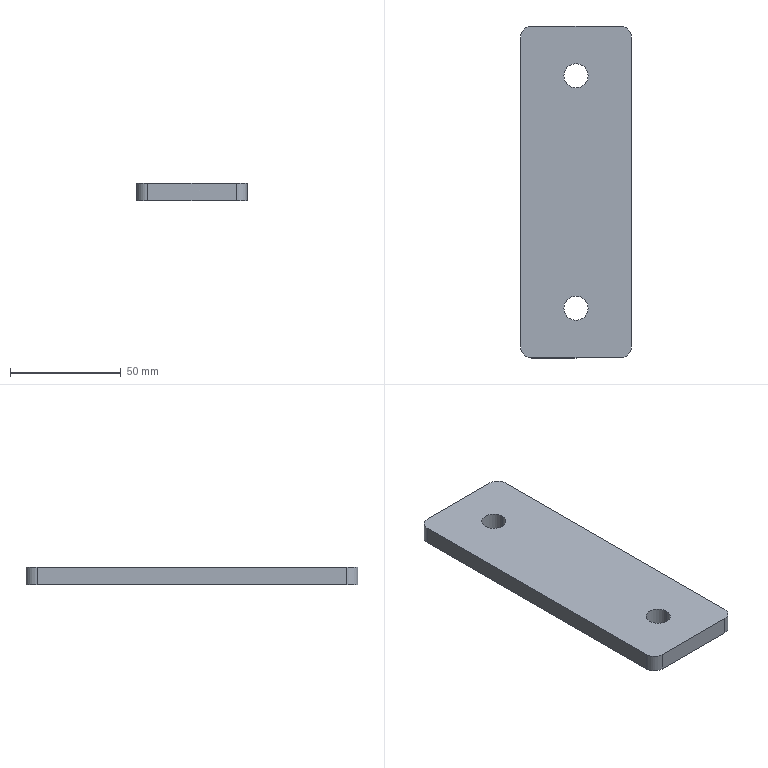Part | SolidWorks | features Extrusion 1, HoleWzd 1 | 1 solid | 14 faces | box 50 x 150 x 8 mm | volume 58308 mm3 | cylinder 8 | plane 6 | commonest cylinder face diameters 10 x4 11 x4
STEP:
#1=CARTESIAN_POINT('',(5.5,52.5,0.));
#2=VERTEX_POINT('',#1);
#3=CARTESIAN_POINT('',(-5.5,52.5,0.));
#4=VERTEX_POINT('',#3);
#5=CARTESIAN_POINT('',(0.,52.5,0.));
#6=DIRECTION('',(0.,0.,-1.));
#7=DIRECTION('',(-1.,0.,0.));
#8=AXIS2_PLACEMENT_3D('',#5,#6,#7);
#9=CIRCLE('',#8,5.5);
#10=EDGE_CURVE('',#2,#4,#9,.T.);
#11=ORIENTED_EDGE('',*,*,#10,.T.);
#12=CARTESIAN_POINT('',(-5.5,52.5,8.));
#13=VERTEX_POINT('',#12);
#14=CARTESIAN_POINT('',(-5.5,52.5,8.));
#15=DIRECTION('',(0.,0.,1.));
#16=VECTOR('',#15,1000.);
#17=LINE('',#14,#16);
#18=EDGE_CURVE('',#4,#13,#17,.T.);
#19=ORIENTED_EDGE('',*,*,#18,.T.);
#20=CARTESIAN_POINT('',(5.5,52.5,8.));
#21=VERTEX_POINT('',#20);
#22=CARTESIAN_POINT('',(0.,52.5,8.));
#23=DIRECTION('',(0.,0.,1.));
#24=DIRECTION('',(1.,0.,0.));
#25=AXIS2_PLACEMENT_3D('',#22,#23,#24);
#26=CIRCLE('',#25,5.5);
#27=EDGE_CURVE('',#13,#21,#26,.T.);
#28=ORIENTED_EDGE('',*,*,#27,.T.);
#29=CARTESIAN_POINT('',(5.5,52.5,8.));
#30=DIRECTION('',(0.,0.,1.));
#31=VECTOR('',#30,1000.);
#32=LINE('',#29,#31);
#33=EDGE_CURVE('',#2,#21,#32,.T.);
#34=ORIENTED_EDGE('',*,*,#33,.F.);
#35=EDGE_LOOP('',(#11,#19,#28,#34));
#36=FACE_OUTER_BOUND('',#35,.T.);
#37=CARTESIAN_POINT('',(0.,52.5,8.));
#38=DIRECTION('',(0.,0.,1.));
#39=DIRECTION('',(1.,0.,0.));
#40=AXIS2_PLACEMENT_3D('',#37,#38,#39);
#41=CYLINDRICAL_SURFACE('',#40,5.5);
#42=ADVANCED_FACE('',(#36),#41,.F.);
#43=CARTESIAN_POINT('',(5.5,-52.5,0.));
#44=VERTEX_POINT('',#43);
#45=CARTESIAN_POINT('',(-5.5,-52.5,0.));
#46=VERTEX_POINT('',#45);
#47=CARTESIAN_POINT('',(0.,-52.5,0.));
#48=DIRECTION('',(0.,0.,-1.));
#49=DIRECTION('',(-1.,0.,0.));
#50=AXIS2_PLACEMENT_3D('',#47,#48,#49);
#51=CIRCLE('',#50,5.5);
#52=EDGE_CURVE('',#44,#46,#51,.T.);
#53=ORIENTED_EDGE('',*,*,#52,.T.);
#54=CARTESIAN_POINT('',(-5.5,-52.5,8.));
#55=VERTEX_POINT('',#54);
#56=CARTESIAN_POINT('',(-5.5,-52.5,8.));
#57=DIRECTION('',(0.,0.,1.));
#58=VECTOR('',#57,1000.);
#59=LINE('',#56,#58);
#60=EDGE_CURVE('',#46,#55,#59,.T.);
#61=ORIENTED_EDGE('',*,*,#60,.T.);
#62=CARTESIAN_POINT('',(5.5,-52.5,8.));
#63=VERTEX_POINT('',#62);
#64=CARTESIAN_POINT('',(0.,-52.5,8.));
#65=DIRECTION('',(0.,0.,1.));
#66=DIRECTION('',(1.,0.,0.));
#67=AXIS2_PLACEMENT_3D('',#64,#65,#66);
#68=CIRCLE('',#67,5.5);
#69=EDGE_CURVE('',#55,#63,#68,.T.);
#70=ORIENTED_EDGE('',*,*,#69,.T.);
#71=CARTESIAN_POINT('',(5.5,-52.5,8.));
#72=DIRECTION('',(0.,0.,1.));
#73=VECTOR('',#72,1000.);
#74=LINE('',#71,#73);
#75=EDGE_CURVE('',#44,#63,#74,.T.);
#76=ORIENTED_EDGE('',*,*,#75,.F.);
#77=EDGE_LOOP('',(#53,#61,#70,#76));
#78=FACE_OUTER_BOUND('',#77,.T.);
#79=CARTESIAN_POINT('',(0.,-52.5,8.));
#80=DIRECTION('',(0.,0.,1.));
#81=DIRECTION('',(1.,0.,0.));
#82=AXIS2_PLACEMENT_3D('',#79,#80,#81);
#83=CYLINDRICAL_SURFACE('',#82,5.5);
#84=ADVANCED_FACE('',(#78),#83,.F.);
#85=CARTESIAN_POINT('',(-25.,-70.,8.));
#86=VERTEX_POINT('',#85);
#87=CARTESIAN_POINT('',(-20.,-75.,8.));
#88=VERTEX_POINT('',#87);
#89=CARTESIAN_POINT('',(-20.,-70.,8.));
#90=DIRECTION('',(0.,0.,1.));
#91=DIRECTION('',(-1.,0.,0.));
#92=AXIS2_PLACEMENT_3D('',#89,#90,#91);
#93=CIRCLE('',#92,5.);
#94=EDGE_CURVE('',#86,#88,#93,.T.);
#95=ORIENTED_EDGE('',*,*,#94,.T.);
#96=CARTESIAN_POINT('',(20.,-75.,8.));
#97=VERTEX_POINT('',#96);
#98=CARTESIAN_POINT('',(20.,-75.,8.));
#99=DIRECTION('',(1.,0.,0.));
#100=VECTOR('',#99,1000.);
#101=LINE('',#98,#100);
#102=EDGE_CURVE('',#88,#97,#101,.T.);
#103=ORIENTED_EDGE('',*,*,#102,.T.);
#104=CARTESIAN_POINT('',(25.,-70.,8.));
#105=VERTEX_POINT('',#104);
#106=CARTESIAN_POINT('',(20.,-70.,8.));
#107=DIRECTION('',(0.,0.,1.));
#108=DIRECTION('',(1.,0.,0.));
#109=AXIS2_PLACEMENT_3D('',#106,#107,#108);
#110=CIRCLE('',#109,5.);
#111=EDGE_CURVE('',#97,#105,#110,.T.);
#112=ORIENTED_EDGE('',*,*,#111,.T.);
#113=CARTESIAN_POINT('',(25.,70.,8.));
#114=VERTEX_POINT('',#113);
#115=CARTESIAN_POINT('',(25.,-70.,8.));
#116=DIRECTION('',(0.,1.,0.));
#117=VECTOR('',#116,1000.);
#118=LINE('',#115,#117);
#119=EDGE_CURVE('',#105,#114,#118,.T.);
#120=ORIENTED_EDGE('',*,*,#119,.T.);
#121=CARTESIAN_POINT('',(20.,75.,8.));
#122=VERTEX_POINT('',#121);
#123=CARTESIAN_POINT('',(20.,70.,8.));
#124=DIRECTION('',(0.,0.,1.));
#125=DIRECTION('',(1.,0.,0.));
#126=AXIS2_PLACEMENT_3D('',#123,#124,#125);
#127=CIRCLE('',#126,5.);
#128=EDGE_CURVE('',#114,#122,#127,.T.);
#129=ORIENTED_EDGE('',*,*,#128,.T.);
#130=CARTESIAN_POINT('',(-20.,75.,8.));
#131=VERTEX_POINT('',#130);
#132=CARTESIAN_POINT('',(20.,75.,8.));
#133=DIRECTION('',(-1.,0.,0.));
#134=VECTOR('',#133,1000.);
#135=LINE('',#132,#134);
#136=EDGE_CURVE('',#122,#131,#135,.T.);
#137=ORIENTED_EDGE('',*,*,#136,.T.);
#138=CARTESIAN_POINT('',(-25.,70.,8.));
#139=VERTEX_POINT('',#138);
#140=CARTESIAN_POINT('',(-20.,70.,8.));
#141=DIRECTION('',(0.,0.,1.));
#142=DIRECTION('',(1.,0.,0.));
#143=AXIS2_PLACEMENT_3D('',#140,#141,#142);
#144=CIRCLE('',#143,5.);
#145=EDGE_CURVE('',#131,#139,#144,.T.);
#146=ORIENTED_EDGE('',*,*,#145,.T.);
#147=CARTESIAN_POINT('',(-25.,-70.,8.));
#148=DIRECTION('',(0.,-1.,0.));
#149=VECTOR('',#148,1000.);
#150=LINE('',#147,#149);
#151=EDGE_CURVE('',#139,#86,#150,.T.);
#152=ORIENTED_EDGE('',*,*,#151,.T.);
#153=EDGE_LOOP('',(#95,#103,#112,#120,#129,#137,#146,#152));
#154=FACE_OUTER_BOUND('',#153,.T.);
#155=CARTESIAN_POINT('',(0.,-52.5,8.));
#156=DIRECTION('',(0.,0.,1.));
#157=DIRECTION('',(1.,0.,0.));
#158=AXIS2_PLACEMENT_3D('',#155,#156,#157);
#159=CIRCLE('',#158,5.5);
#160=EDGE_CURVE('',#63,#55,#159,.T.);
#161=ORIENTED_EDGE('',*,*,#160,.F.);
#162=ORIENTED_EDGE('',*,*,#69,.F.);
#163=EDGE_LOOP('',(#161,#162));
#164=FACE_BOUND('',#163,.T.);
#165=CARTESIAN_POINT('',(0.,52.5,8.));
#166=DIRECTION('',(0.,0.,1.));
#167=DIRECTION('',(1.,0.,0.));
#168=AXIS2_PLACEMENT_3D('',#165,#166,#167);
#169=CIRCLE('',#168,5.5);
#170=EDGE_CURVE('',#21,#13,#169,.T.);
#171=ORIENTED_EDGE('',*,*,#170,.F.);
#172=ORIENTED_EDGE('',*,*,#27,.F.);
#173=EDGE_LOOP('',(#171,#172));
#174=FACE_BOUND('',#173,.T.);
#175=CARTESIAN_POINT('',(-20.,-70.,8.));
#176=DIRECTION('',(0.,0.,-1.));
#177=DIRECTION('',(-1.,0.,0.));
#178=AXIS2_PLACEMENT_3D('',#175,#176,#177);
#179=PLANE('',#178);
#180=ADVANCED_FACE('',(#154,#164,#174),#179,.F.);
#181=CARTESIAN_POINT('',(-25.,-70.,0.));
#182=VERTEX_POINT('',#181);
#183=CARTESIAN_POINT('',(-20.,-75.,0.));
#184=VERTEX_POINT('',#183);
#185=CARTESIAN_POINT('',(-20.,-70.,0.));
#186=DIRECTION('',(0.,0.,1.));
#187=DIRECTION('',(-1.,0.,0.));
#188=AXIS2_PLACEMENT_3D('',#185,#186,#187);
#189=CIRCLE('',#188,5.);
#190=EDGE_CURVE('',#182,#184,#189,.T.);
#191=ORIENTED_EDGE('',*,*,#190,.T.);
#192=CARTESIAN_POINT('',(-20.,-75.,8.));
#193=DIRECTION('',(0.,0.,-1.));
#194=VECTOR('',#193,1000.);
#195=LINE('',#192,#194);
#196=EDGE_CURVE('',#88,#184,#195,.T.);
#197=ORIENTED_EDGE('',*,*,#196,.F.);
#198=ORIENTED_EDGE('',*,*,#94,.F.);
#199=CARTESIAN_POINT('',(-25.,-70.,8.));
#200=DIRECTION('',(0.,0.,-1.));
#201=VECTOR('',#200,1000.);
#202=LINE('',#199,#201);
#203=EDGE_CURVE('',#86,#182,#202,.T.);
#204=ORIENTED_EDGE('',*,*,#203,.T.);
#205=EDGE_LOOP('',(#191,#197,#198,#204));
#206=FACE_OUTER_BOUND('',#205,.T.);
#207=CARTESIAN_POINT('',(-20.,-70.,8.));
#208=DIRECTION('',(0.,0.,-1.));
#209=DIRECTION('',(-1.,0.,0.));
#210=AXIS2_PLACEMENT_3D('',#207,#208,#209);
#211=CYLINDRICAL_SURFACE('',#210,5.);
#212=ADVANCED_FACE('',(#206),#211,.T.);
#213=CARTESIAN_POINT('',(20.,-75.,0.));
#214=VERTEX_POINT('',#213);
#215=CARTESIAN_POINT('',(20.,-75.,0.));
#216=DIRECTION('',(1.,0.,0.));
#217=VECTOR('',#216,1000.);
#218=LINE('',#215,#217);
#219=EDGE_CURVE('',#184,#214,#218,.T.);
#220=ORIENTED_EDGE('',*,*,#219,.T.);
#221=CARTESIAN_POINT('',(20.,-75.,8.));
#222=DIRECTION('',(0.,0.,-1.));
#223=VECTOR('',#222,1000.);
#224=LINE('',#221,#223);
#225=EDGE_CURVE('',#97,#214,#224,.T.);
#226=ORIENTED_EDGE('',*,*,#225,.F.);
#227=ORIENTED_EDGE('',*,*,#102,.F.);
#228=ORIENTED_EDGE('',*,*,#196,.T.);
#229=EDGE_LOOP('',(#220,#226,#227,#228));
#230=FACE_OUTER_BOUND('',#229,.T.);
#231=CARTESIAN_POINT('',(20.,-75.,8.));
#232=DIRECTION('',(0.,1.,0.));
#233=DIRECTION('',(-1.,0.,0.));
#234=AXIS2_PLACEMENT_3D('',#231,#232,#233);
#235=PLANE('',#234);
#236=ADVANCED_FACE('',(#230),#235,.F.);
#237=CARTESIAN_POINT('',(25.,-70.,0.));
#238=VERTEX_POINT('',#237);
#239=CARTESIAN_POINT('',(20.,-70.,0.));
#240=DIRECTION('',(0.,0.,1.));
#241=DIRECTION('',(1.,0.,0.));
#242=AXIS2_PLACEMENT_3D('',#239,#240,#241);
#243=CIRCLE('',#242,5.);
#244=EDGE_CURVE('',#214,#238,#243,.T.);
#245=ORIENTED_EDGE('',*,*,#244,.T.);
#246=CARTESIAN_POINT('',(25.,-70.,8.));
#247=DIRECTION('',(0.,0.,-1.));
#248=VECTOR('',#247,1000.);
#249=LINE('',#246,#248);
#250=EDGE_CURVE('',#105,#238,#249,.T.);
#251=ORIENTED_EDGE('',*,*,#250,.F.);
#252=ORIENTED_EDGE('',*,*,#111,.F.);
#253=ORIENTED_EDGE('',*,*,#225,.T.);
#254=EDGE_LOOP('',(#245,#251,#252,#253));
#255=FACE_OUTER_BOUND('',#254,.T.);
#256=CARTESIAN_POINT('',(20.,-70.,8.));
#257=DIRECTION('',(0.,0.,-1.));
#258=DIRECTION('',(-1.,0.,0.));
#259=AXIS2_PLACEMENT_3D('',#256,#257,#258);
#260=CYLINDRICAL_SURFACE('',#259,5.);
#261=ADVANCED_FACE('',(#255),#260,.T.);
#262=CARTESIAN_POINT('',(25.,70.,0.));
#263=VERTEX_POINT('',#262);
#264=CARTESIAN_POINT('',(25.,-70.,0.));
#265=DIRECTION('',(0.,1.,0.));
#266=VECTOR('',#265,1000.);
#267=LINE('',#264,#266);
#268=EDGE_CURVE('',#238,#263,#267,.T.);
#269=ORIENTED_EDGE('',*,*,#268,.T.);
#270=CARTESIAN_POINT('',(25.,70.,8.));
#271=DIRECTION('',(0.,0.,-1.));
#272=VECTOR('',#271,1000.);
#273=LINE('',#270,#272);
#274=EDGE_CURVE('',#114,#263,#273,.T.);
#275=ORIENTED_EDGE('',*,*,#274,.F.);
#276=ORIENTED_EDGE('',*,*,#119,.F.);
#277=ORIENTED_EDGE('',*,*,#250,.T.);
#278=EDGE_LOOP('',(#269,#275,#276,#277));
#279=FACE_OUTER_BOUND('',#278,.T.);
#280=CARTESIAN_POINT('',(25.,-70.,8.));
#281=DIRECTION('',(-1.,0.,0.));
#282=DIRECTION('',(0.,0.,1.));
#283=AXIS2_PLACEMENT_3D('',#280,#281,#282);
#284=PLANE('',#283);
#285=ADVANCED_FACE('',(#279),#284,.F.);
#286=CARTESIAN_POINT('',(20.,75.,0.));
#287=VERTEX_POINT('',#286);
#288=CARTESIAN_POINT('',(20.,70.,0.));
#289=DIRECTION('',(0.,0.,1.));
#290=DIRECTION('',(1.,0.,0.));
#291=AXIS2_PLACEMENT_3D('',#288,#289,#290);
#292=CIRCLE('',#291,5.);
#293=EDGE_CURVE('',#263,#287,#292,.T.);
#294=ORIENTED_EDGE('',*,*,#293,.T.);
#295=CARTESIAN_POINT('',(20.,75.,8.));
#296=DIRECTION('',(0.,0.,-1.));
#297=VECTOR('',#296,1000.);
#298=LINE('',#295,#297);
#299=EDGE_CURVE('',#122,#287,#298,.T.);
#300=ORIENTED_EDGE('',*,*,#299,.F.);
#301=ORIENTED_EDGE('',*,*,#128,.F.);
#302=ORIENTED_EDGE('',*,*,#274,.T.);
#303=EDGE_LOOP('',(#294,#300,#301,#302));
#304=FACE_OUTER_BOUND('',#303,.T.);
#305=CARTESIAN_POINT('',(20.,70.,8.));
#306=DIRECTION('',(0.,0.,-1.));
#307=DIRECTION('',(-1.,0.,0.));
#308=AXIS2_PLACEMENT_3D('',#305,#306,#307);
#309=CYLINDRICAL_SURFACE('',#308,5.);
#310=ADVANCED_FACE('',(#304),#309,.T.);
#311=CARTESIAN_POINT('',(-20.,75.,0.));
#312=VERTEX_POINT('',#311);
#313=CARTESIAN_POINT('',(20.,75.,0.));
#314=DIRECTION('',(-1.,0.,0.));
#315=VECTOR('',#314,1000.);
#316=LINE('',#313,#315);
#317=EDGE_CURVE('',#287,#312,#316,.T.);
#318=ORIENTED_EDGE('',*,*,#317,.T.);
#319=CARTESIAN_POINT('',(-20.,75.,8.));
#320=DIRECTION('',(0.,0.,-1.));
#321=VECTOR('',#320,1000.);
#322=LINE('',#319,#321);
#323=EDGE_CURVE('',#131,#312,#322,.T.);
#324=ORIENTED_EDGE('',*,*,#323,.F.);
#325=ORIENTED_EDGE('',*,*,#136,.F.);
#326=ORIENTED_EDGE('',*,*,#299,.T.);
#327=EDGE_LOOP('',(#318,#324,#325,#326));
#328=FACE_OUTER_BOUND('',#327,.T.);
#329=CARTESIAN_POINT('',(20.,75.,8.));
#330=DIRECTION('',(0.,-1.,0.));
#331=DIRECTION('',(0.,0.,-1.));
#332=AXIS2_PLACEMENT_3D('',#329,#330,#331);
#333=PLANE('',#332);
#334=ADVANCED_FACE('',(#328),#333,.F.);
#335=CARTESIAN_POINT('',(-25.,70.,0.));
#336=VERTEX_POINT('',#335);
#337=CARTESIAN_POINT('',(-20.,70.,0.));
#338=DIRECTION('',(0.,0.,1.));
#339=DIRECTION('',(1.,0.,0.));
#340=AXIS2_PLACEMENT_3D('',#337,#338,#339);
#341=CIRCLE('',#340,5.);
#342=EDGE_CURVE('',#312,#336,#341,.T.);
#343=ORIENTED_EDGE('',*,*,#342,.T.);
#344=CARTESIAN_POINT('',(-25.,70.,8.));
#345=DIRECTION('',(0.,0.,-1.));
#346=VECTOR('',#345,1000.);
#347=LINE('',#344,#346);
#348=EDGE_CURVE('',#139,#336,#347,.T.);
#349=ORIENTED_EDGE('',*,*,#348,.F.);
#350=ORIENTED_EDGE('',*,*,#145,.F.);
#351=ORIENTED_EDGE('',*,*,#323,.T.);
#352=EDGE_LOOP('',(#343,#349,#350,#351));
#353=FACE_OUTER_BOUND('',#352,.T.);
#354=CARTESIAN_POINT('',(-20.,70.,8.));
#355=DIRECTION('',(0.,0.,-1.));
#356=DIRECTION('',(-1.,0.,0.));
#357=AXIS2_PLACEMENT_3D('',#354,#355,#356);
#358=CYLINDRICAL_SURFACE('',#357,5.);
#359=ADVANCED_FACE('',(#353),#358,.T.);
#360=CARTESIAN_POINT('',(-25.,-70.,0.));
#361=DIRECTION('',(0.,-1.,0.));
#362=VECTOR('',#361,1000.);
#363=LINE('',#360,#362);
#364=EDGE_CURVE('',#336,#182,#363,.T.);
#365=ORIENTED_EDGE('',*,*,#364,.T.);
#366=ORIENTED_EDGE('',*,*,#203,.F.);
#367=ORIENTED_EDGE('',*,*,#151,.F.);
#368=ORIENTED_EDGE('',*,*,#348,.T.);
#369=EDGE_LOOP('',(#365,#366,#367,#368));
#370=FACE_OUTER_BOUND('',#369,.T.);
#371=CARTESIAN_POINT('',(-25.,-70.,8.));
#372=DIRECTION('',(1.,0.,0.));
#373=DIRECTION('',(0.,1.,0.));
#374=AXIS2_PLACEMENT_3D('',#371,#372,#373);
#375=PLANE('',#374);
#376=ADVANCED_FACE('',(#370),#375,.F.);
#377=ORIENTED_EDGE('',*,*,#10,.F.);
#378=CARTESIAN_POINT('',(0.,52.5,0.));
#379=DIRECTION('',(0.,0.,-1.));
#380=DIRECTION('',(-1.,0.,0.));
#381=AXIS2_PLACEMENT_3D('',#378,#379,#380);
#382=CIRCLE('',#381,5.5);
#383=EDGE_CURVE('',#4,#2,#382,.T.);
#384=ORIENTED_EDGE('',*,*,#383,.F.);
#385=EDGE_LOOP('',(#377,#384));
#386=FACE_BOUND('',#385,.T.);
#387=ORIENTED_EDGE('',*,*,#52,.F.);
#388=CARTESIAN_POINT('',(0.,-52.5,0.));
#389=DIRECTION('',(0.,0.,-1.));
#390=DIRECTION('',(-1.,0.,0.));
#391=AXIS2_PLACEMENT_3D('',#388,#389,#390);
#392=CIRCLE('',#391,5.5);
#393=EDGE_CURVE('',#46,#44,#392,.T.);
#394=ORIENTED_EDGE('',*,*,#393,.F.);
#395=EDGE_LOOP('',(#387,#394));
#396=FACE_BOUND('',#395,.T.);
#397=ORIENTED_EDGE('',*,*,#190,.F.);
#398=ORIENTED_EDGE('',*,*,#364,.F.);
#399=ORIENTED_EDGE('',*,*,#342,.F.);
#400=ORIENTED_EDGE('',*,*,#317,.F.);
#401=ORIENTED_EDGE('',*,*,#293,.F.);
#402=ORIENTED_EDGE('',*,*,#268,.F.);
#403=ORIENTED_EDGE('',*,*,#244,.F.);
#404=ORIENTED_EDGE('',*,*,#219,.F.);
#405=EDGE_LOOP('',(#397,#398,#399,#400,#401,#402,#403,#404));
#406=FACE_OUTER_BOUND('',#405,.T.);
#407=CARTESIAN_POINT('',(-20.,-70.,0.));
#408=DIRECTION('',(0.,0.,-1.));
#409=DIRECTION('',(-1.,0.,0.));
#410=AXIS2_PLACEMENT_3D('',#407,#408,#409);
#411=PLANE('',#410);
#412=ADVANCED_FACE('',(#386,#396,#406),#411,.T.);
#413=ORIENTED_EDGE('',*,*,#60,.F.);
#414=ORIENTED_EDGE('',*,*,#393,.T.);
#415=ORIENTED_EDGE('',*,*,#75,.T.);
#416=ORIENTED_EDGE('',*,*,#160,.T.);
#417=EDGE_LOOP('',(#413,#414,#415,#416));
#418=FACE_OUTER_BOUND('',#417,.T.);
#419=CARTESIAN_POINT('',(0.,-52.5,8.));
#420=DIRECTION('',(0.,0.,1.));
#421=DIRECTION('',(1.,0.,0.));
#422=AXIS2_PLACEMENT_3D('',#419,#420,#421);
#423=CYLINDRICAL_SURFACE('',#422,5.5);
#424=ADVANCED_FACE('',(#418),#423,.F.);
#425=ORIENTED_EDGE('',*,*,#18,.F.);
#426=ORIENTED_EDGE('',*,*,#383,.T.);
#427=ORIENTED_EDGE('',*,*,#33,.T.);
#428=ORIENTED_EDGE('',*,*,#170,.T.);
#429=EDGE_LOOP('',(#425,#426,#427,#428));
#430=FACE_OUTER_BOUND('',#429,.T.);
#431=CARTESIAN_POINT('',(0.,52.5,8.));
#432=DIRECTION('',(0.,0.,1.));
#433=DIRECTION('',(1.,0.,0.));
#434=AXIS2_PLACEMENT_3D('',#431,#432,#433);
#435=CYLINDRICAL_SURFACE('',#434,5.5);
#436=ADVANCED_FACE('',(#430),#435,.F.);
#437=CLOSED_SHELL('',(#42,#84,#180,#212,#236,#261,#285,#310,#334,#359,#376,#412,#424,#436));
#438=MANIFOLD_SOLID_BREP('',#437);
#439=CARTESIAN_POINT('',(0.,0.,0.));
#440=DIRECTION('',(0.,0.,1.));
#441=DIRECTION('',(1.,0.,0.));
#442=AXIS2_PLACEMENT_3D('',#439,#440,#441);
#443=(LENGTH_UNIT()NAMED_UNIT(*)SI_UNIT(.MILLI.,.METRE.));
#444=UNCERTAINTY_MEASURE_WITH_UNIT(LENGTH_MEASURE(0.00001),#443,'','');
#445=(NAMED_UNIT(*)PLANE_ANGLE_UNIT()SI_UNIT($,.RADIAN.));
#446=(NAMED_UNIT(*)SI_UNIT($,.STERADIAN.)SOLID_ANGLE_UNIT());
#447=(GEOMETRIC_REPRESENTATION_CONTEXT(3)GLOBAL_UNCERTAINTY_ASSIGNED_CONTEXT((#444))GLOBAL_UNIT_ASSIGNED_CONTEXT((#443,#445,#446))REPRESENTATION_CONTEXT('',''));
#448=ADVANCED_BREP_SHAPE_REPRESENTATION('',(#438,#442),#447);